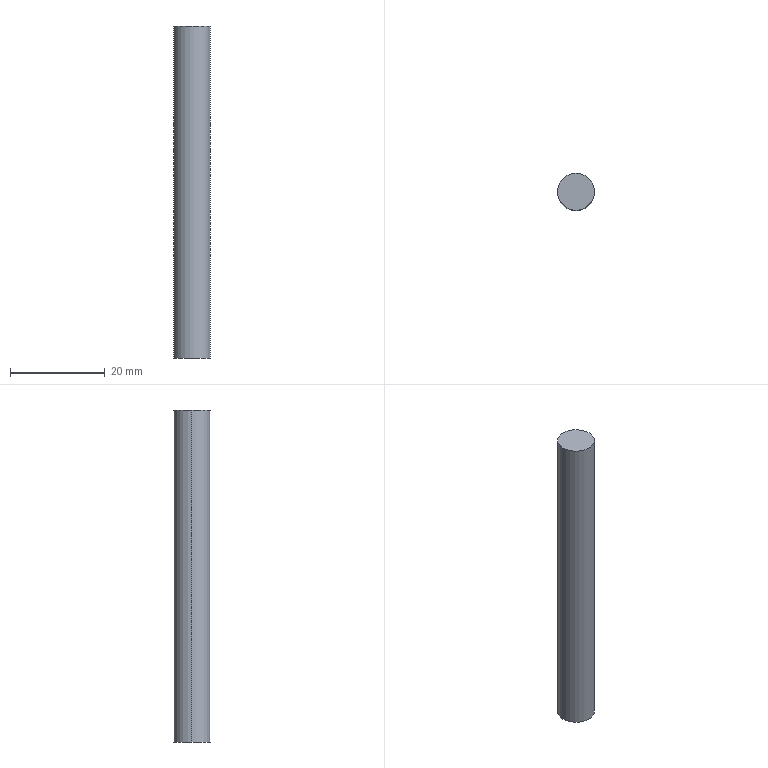Part | SolidWorks | features MirrorStock 1 | 1 solid | 4 faces | box 7.8 x 7.8 x 70 mm | volume 3345 mm3 | cylinder 2 | plane 2 | commonest cylinder face diameters 7.8 x2
STEP:
#1=CARTESIAN_POINT('',(4.1,-61.753,-70.));
#2=VERTEX_POINT('',#1);
#3=CARTESIAN_POINT('',(11.9,-61.753,-70.));
#4=VERTEX_POINT('',#3);
#5=CARTESIAN_POINT('',(8.,-61.753,-70.));
#6=DIRECTION('',(0.,0.,1.));
#7=DIRECTION('',(1.,0.,0.));
#8=AXIS2_PLACEMENT_3D('',#5,#6,#7);
#9=CIRCLE('',#8,3.9);
#10=EDGE_CURVE('',#2,#4,#9,.T.);
#11=ORIENTED_EDGE('',*,*,#10,.T.);
#12=CARTESIAN_POINT('',(11.9,-61.753,0.));
#13=VERTEX_POINT('',#12);
#14=CARTESIAN_POINT('',(11.9,-61.753,-70.));
#15=DIRECTION('',(0.,0.,1.));
#16=VECTOR('',#15,1000.);
#17=LINE('',#14,#16);
#18=EDGE_CURVE('',#4,#13,#17,.T.);
#19=ORIENTED_EDGE('',*,*,#18,.T.);
#20=CARTESIAN_POINT('',(4.1,-61.753,0.));
#21=VERTEX_POINT('',#20);
#22=CARTESIAN_POINT('',(8.,-61.753,0.));
#23=DIRECTION('',(0.,0.,1.));
#24=DIRECTION('',(1.,0.,0.));
#25=AXIS2_PLACEMENT_3D('',#22,#23,#24);
#26=CIRCLE('',#25,3.9);
#27=EDGE_CURVE('',#21,#13,#26,.T.);
#28=ORIENTED_EDGE('',*,*,#27,.F.);
#29=CARTESIAN_POINT('',(4.1,-61.753,-70.));
#30=DIRECTION('',(0.,0.,1.));
#31=VECTOR('',#30,1000.);
#32=LINE('',#29,#31);
#33=EDGE_CURVE('',#2,#21,#32,.T.);
#34=ORIENTED_EDGE('',*,*,#33,.F.);
#35=EDGE_LOOP('',(#11,#19,#28,#34));
#36=FACE_OUTER_BOUND('',#35,.T.);
#37=CARTESIAN_POINT('',(8.,-61.753,-70.));
#38=DIRECTION('',(0.,0.,1.));
#39=DIRECTION('',(-1.,0.,0.));
#40=AXIS2_PLACEMENT_3D('',#37,#38,#39);
#41=CYLINDRICAL_SURFACE('',#40,3.9);
#42=ADVANCED_FACE('',(#36),#41,.T.);
#43=ORIENTED_EDGE('',*,*,#18,.F.);
#44=CARTESIAN_POINT('',(8.,-61.753,-70.));
#45=DIRECTION('',(0.,0.,1.));
#46=DIRECTION('',(1.,0.,0.));
#47=AXIS2_PLACEMENT_3D('',#44,#45,#46);
#48=CIRCLE('',#47,3.9);
#49=EDGE_CURVE('',#4,#2,#48,.T.);
#50=ORIENTED_EDGE('',*,*,#49,.T.);
#51=ORIENTED_EDGE('',*,*,#33,.T.);
#52=CARTESIAN_POINT('',(8.,-61.753,0.));
#53=DIRECTION('',(0.,0.,1.));
#54=DIRECTION('',(1.,0.,0.));
#55=AXIS2_PLACEMENT_3D('',#52,#53,#54);
#56=CIRCLE('',#55,3.9);
#57=EDGE_CURVE('',#13,#21,#56,.T.);
#58=ORIENTED_EDGE('',*,*,#57,.F.);
#59=EDGE_LOOP('',(#43,#50,#51,#58));
#60=FACE_OUTER_BOUND('',#59,.T.);
#61=CARTESIAN_POINT('',(8.,-61.753,-70.));
#62=DIRECTION('',(0.,0.,1.));
#63=DIRECTION('',(-1.,0.,0.));
#64=AXIS2_PLACEMENT_3D('',#61,#62,#63);
#65=CYLINDRICAL_SURFACE('',#64,3.9);
#66=ADVANCED_FACE('',(#60),#65,.T.);
#67=ORIENTED_EDGE('',*,*,#10,.F.);
#68=ORIENTED_EDGE('',*,*,#49,.F.);
#69=EDGE_LOOP('',(#67,#68));
#70=FACE_OUTER_BOUND('',#69,.T.);
#71=CARTESIAN_POINT('',(8.,-61.753,-70.));
#72=DIRECTION('',(0.,0.,-1.));
#73=DIRECTION('',(1.,0.,0.));
#74=AXIS2_PLACEMENT_3D('',#71,#72,#73);
#75=PLANE('',#74);
#76=ADVANCED_FACE('',(#70),#75,.T.);
#77=ORIENTED_EDGE('',*,*,#27,.T.);
#78=ORIENTED_EDGE('',*,*,#57,.T.);
#79=EDGE_LOOP('',(#77,#78));
#80=FACE_OUTER_BOUND('',#79,.T.);
#81=CARTESIAN_POINT('',(8.,-61.753,0.));
#82=DIRECTION('',(0.,0.,-1.));
#83=DIRECTION('',(1.,0.,0.));
#84=AXIS2_PLACEMENT_3D('',#81,#82,#83);
#85=PLANE('',#84);
#86=ADVANCED_FACE('',(#80),#85,.F.);
#87=CLOSED_SHELL('',(#42,#66,#76,#86));
#88=MANIFOLD_SOLID_BREP('',#87);
#89=CARTESIAN_POINT('',(0.,0.,0.));
#90=DIRECTION('',(0.,0.,1.));
#91=DIRECTION('',(1.,0.,0.));
#92=AXIS2_PLACEMENT_3D('',#89,#90,#91);
#93=(LENGTH_UNIT()NAMED_UNIT(*)SI_UNIT(.MILLI.,.METRE.));
#94=UNCERTAINTY_MEASURE_WITH_UNIT(LENGTH_MEASURE(0.00001),#93,'','');
#95=(NAMED_UNIT(*)PLANE_ANGLE_UNIT()SI_UNIT($,.RADIAN.));
#96=(NAMED_UNIT(*)SI_UNIT($,.STERADIAN.)SOLID_ANGLE_UNIT());
#97=(GEOMETRIC_REPRESENTATION_CONTEXT(3)GLOBAL_UNCERTAINTY_ASSIGNED_CONTEXT((#94))GLOBAL_UNIT_ASSIGNED_CONTEXT((#93,#95,#96))REPRESENTATION_CONTEXT('',''));
#98=ADVANCED_BREP_SHAPE_REPRESENTATION('',(#88,#92),#97);